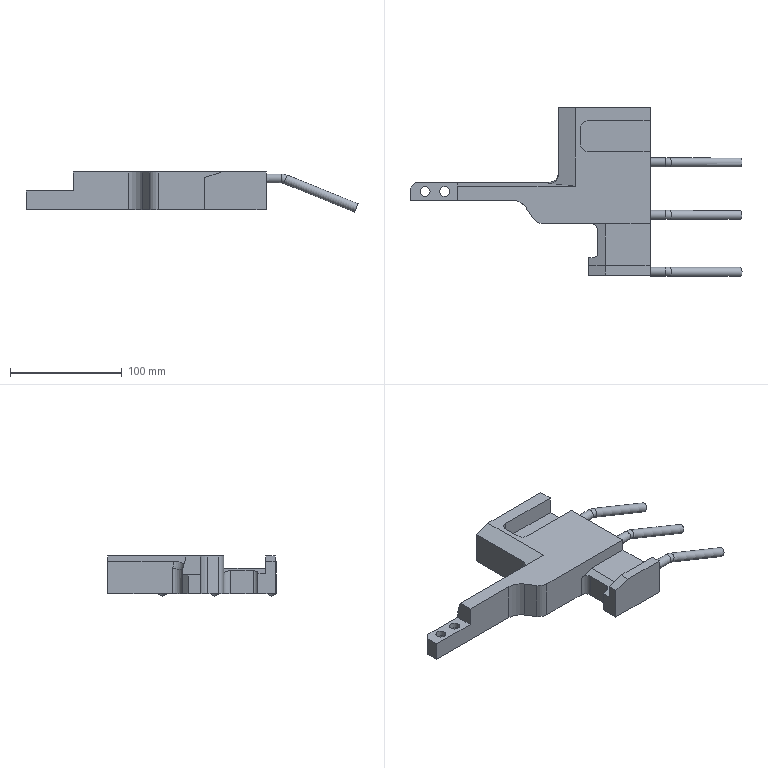Part | STEP file | gslz 2016.10.28-13_id374_x_t | 1 solid | 55 faces | box 297.336 x 150.996 x 35.855 mm | volume 404326 mm3 | plane 34 | cylinder 18 | torus 3 | commonest cylinder face diameters 8 x7 12 x3 9 x2 14 x2 18 x2 20 x1